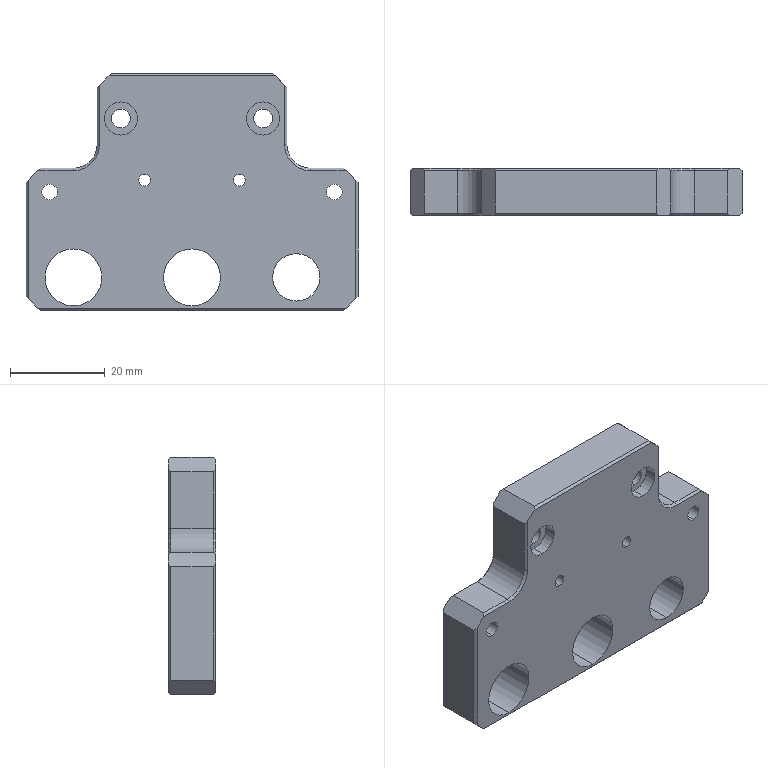Part | SolidWorks | features ICE 5, Chamfer 3, HoleWzd 2, Cut 1, Extrusion 1, Fillet 1 | 1 solid | 68 faces | box 70 x 10 x 50 mm | volume 24960 mm3 | plane 36 | cylinder 28 | cone 4 | commonest cylinder face diameters 7 x8 2.5 x4 3.3 x4 4 x4 10 x4 12 x4